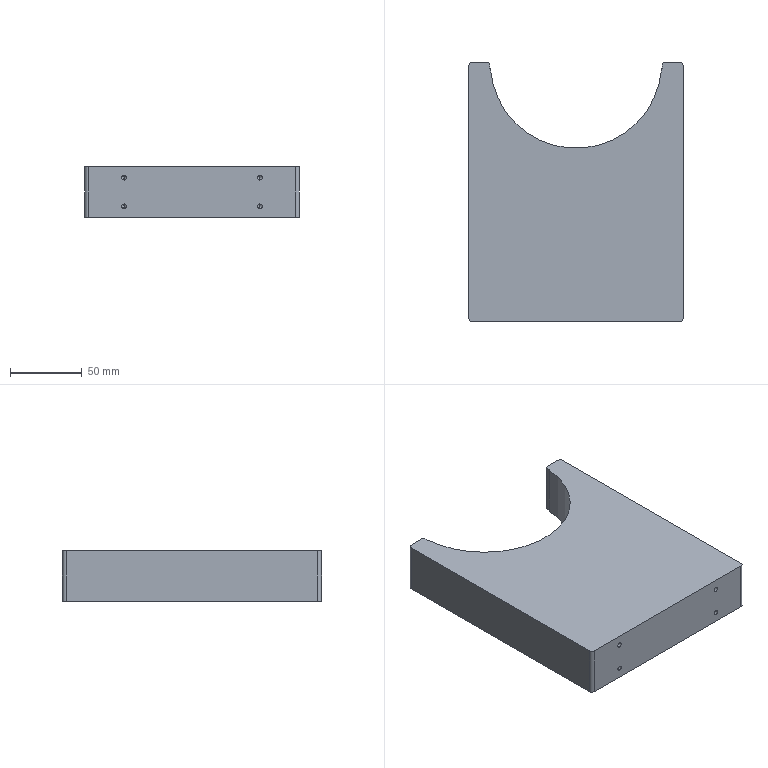Part | SolidWorks | features HoleWzd 2, ICE 2, Chamfer 1, Extrusion 1, Fillet 1 | 1 solid | 42 faces | box 150 x 181 x 35 mm | volume 751527 mm3 | cylinder 19 | cone 12 | plane 11 | commonest cylinder face diameters 3.3 x12 5 x4 120.9 x2 119.9 x1
STEP:
#1=CARTESIAN_POINT('',(-47.5,-75.5,11.65));
#2=VERTEX_POINT('',#1);
#3=CARTESIAN_POINT('',(-47.5,-75.5,8.35));
#4=VERTEX_POINT('',#3);
#5=CARTESIAN_POINT('',(-47.5,-75.5,10.));
#6=DIRECTION('',(0.,-1.,0.));
#7=DIRECTION('',(0.,0.,-1.));
#8=AXIS2_PLACEMENT_3D('',#5,#6,#7);
#9=CIRCLE('',#8,1.65);
#10=EDGE_CURVE('',#2,#4,#9,.T.);
#11=ORIENTED_EDGE('',*,*,#10,.F.);
#12=CARTESIAN_POINT('',(-47.5,-90.5,11.65));
#13=VERTEX_POINT('',#12);
#14=CARTESIAN_POINT('',(-47.5,-90.5,11.65));
#15=DIRECTION('',(0.,-1.,0.));
#16=VECTOR('',#15,1000.);
#17=LINE('',#14,#16);
#18=EDGE_CURVE('',#2,#13,#17,.T.);
#19=ORIENTED_EDGE('',*,*,#18,.T.);
#20=CARTESIAN_POINT('',(-47.5,-90.5,8.35));
#21=VERTEX_POINT('',#20);
#22=CARTESIAN_POINT('',(-47.5,-90.5,10.));
#23=DIRECTION('',(0.,-1.,0.));
#24=DIRECTION('',(0.,0.,-1.));
#25=AXIS2_PLACEMENT_3D('',#22,#23,#24);
#26=CIRCLE('',#25,1.65);
#27=EDGE_CURVE('',#13,#21,#26,.T.);
#28=ORIENTED_EDGE('',*,*,#27,.T.);
#29=CARTESIAN_POINT('',(-47.5,-90.5,8.35));
#30=DIRECTION('',(0.,-1.,0.));
#31=VECTOR('',#30,1000.);
#32=LINE('',#29,#31);
#33=EDGE_CURVE('',#4,#21,#32,.T.);
#34=ORIENTED_EDGE('',*,*,#33,.F.);
#35=EDGE_LOOP('',(#11,#19,#28,#34));
#36=FACE_OUTER_BOUND('',#35,.T.);
#37=CARTESIAN_POINT('',(-47.5,-90.5,10.));
#38=DIRECTION('',(0.,-1.,0.));
#39=DIRECTION('',(0.,0.,-1.));
#40=AXIS2_PLACEMENT_3D('',#37,#38,#39);
#41=CYLINDRICAL_SURFACE('',#40,1.65);
#42=ADVANCED_FACE('',(#36),#41,.F.);
#43=CARTESIAN_POINT('',(-47.5,-74.509,10.));
#44=VERTEX_POINT('',#43);
#45=CARTESIAN_POINT('',(-47.5,-75.5,8.35));
#46=DIRECTION('',(0.,-0.515,-0.8572));
#47=VECTOR('',#46,1000.);
#48=LINE('',#45,#47);
#49=EDGE_CURVE('',#44,#4,#48,.T.);
#50=ORIENTED_EDGE('',*,*,#49,.F.);
#51=CARTESIAN_POINT('',(-47.5,-75.5,11.65));
#52=DIRECTION('',(0.,-0.515,0.8572));
#53=VECTOR('',#52,1000.);
#54=LINE('',#51,#53);
#55=EDGE_CURVE('',#44,#2,#54,.T.);
#56=ORIENTED_EDGE('',*,*,#55,.T.);
#57=ORIENTED_EDGE('',*,*,#10,.T.);
#58=EDGE_LOOP('',(#50,#56,#57));
#59=FACE_OUTER_BOUND('',#58,.T.);
#60=CARTESIAN_POINT('',(-47.5,-75.5,10.));
#61=DIRECTION('',(0.,-1.,0.));
#62=DIRECTION('',(0.,0.,-1.));
#63=AXIS2_PLACEMENT_3D('',#60,#61,#62);
#64=CONICAL_SURFACE('',#63,1.65,1.03);
#65=ADVANCED_FACE('',(#59),#64,.F.);
#66=CARTESIAN_POINT('',(-47.5,-75.5,-8.35));
#67=VERTEX_POINT('',#66);
#68=CARTESIAN_POINT('',(-47.5,-75.5,-11.65));
#69=VERTEX_POINT('',#68);
#70=CARTESIAN_POINT('',(-47.5,-75.5,-10.));
#71=DIRECTION('',(0.,-1.,0.));
#72=DIRECTION('',(0.,0.,-1.));
#73=AXIS2_PLACEMENT_3D('',#70,#71,#72);
#74=CIRCLE('',#73,1.65);
#75=EDGE_CURVE('',#67,#69,#74,.T.);
#76=ORIENTED_EDGE('',*,*,#75,.F.);
#77=CARTESIAN_POINT('',(-47.5,-90.5,-8.35));
#78=VERTEX_POINT('',#77);
#79=CARTESIAN_POINT('',(-47.5,-90.5,-8.35));
#80=DIRECTION('',(0.,-1.,0.));
#81=VECTOR('',#80,1000.);
#82=LINE('',#79,#81);
#83=EDGE_CURVE('',#67,#78,#82,.T.);
#84=ORIENTED_EDGE('',*,*,#83,.T.);
#85=CARTESIAN_POINT('',(-47.5,-90.5,-11.65));
#86=VERTEX_POINT('',#85);
#87=CARTESIAN_POINT('',(-47.5,-90.5,-10.));
#88=DIRECTION('',(0.,-1.,0.));
#89=DIRECTION('',(0.,0.,-1.));
#90=AXIS2_PLACEMENT_3D('',#87,#88,#89);
#91=CIRCLE('',#90,1.65);
#92=EDGE_CURVE('',#78,#86,#91,.T.);
#93=ORIENTED_EDGE('',*,*,#92,.T.);
#94=CARTESIAN_POINT('',(-47.5,-90.5,-11.65));
#95=DIRECTION('',(0.,-1.,0.));
#96=VECTOR('',#95,1000.);
#97=LINE('',#94,#96);
#98=EDGE_CURVE('',#69,#86,#97,.T.);
#99=ORIENTED_EDGE('',*,*,#98,.F.);
#100=EDGE_LOOP('',(#76,#84,#93,#99));
#101=FACE_OUTER_BOUND('',#100,.T.);
#102=CARTESIAN_POINT('',(-47.5,-90.5,-10.));
#103=DIRECTION('',(0.,-1.,0.));
#104=DIRECTION('',(0.,0.,-1.));
#105=AXIS2_PLACEMENT_3D('',#102,#103,#104);
#106=CYLINDRICAL_SURFACE('',#105,1.65);
#107=ADVANCED_FACE('',(#101),#106,.F.);
#108=CARTESIAN_POINT('',(-47.5,-74.509,-10.));
#109=VERTEX_POINT('',#108);
#110=CARTESIAN_POINT('',(-47.5,-75.5,-11.65));
#111=DIRECTION('',(0.,-0.515,-0.8572));
#112=VECTOR('',#111,1000.);
#113=LINE('',#110,#112);
#114=EDGE_CURVE('',#109,#69,#113,.T.);
#115=ORIENTED_EDGE('',*,*,#114,.F.);
#116=CARTESIAN_POINT('',(-47.5,-75.5,-8.35));
#117=DIRECTION('',(0.,-0.515,0.8572));
#118=VECTOR('',#117,1000.);
#119=LINE('',#116,#118);
#120=EDGE_CURVE('',#109,#67,#119,.T.);
#121=ORIENTED_EDGE('',*,*,#120,.T.);
#122=ORIENTED_EDGE('',*,*,#75,.T.);
#123=EDGE_LOOP('',(#115,#121,#122));
#124=FACE_OUTER_BOUND('',#123,.T.);
#125=CARTESIAN_POINT('',(-47.5,-75.5,-10.));
#126=DIRECTION('',(0.,-1.,0.));
#127=DIRECTION('',(0.,0.,-1.));
#128=AXIS2_PLACEMENT_3D('',#125,#126,#127);
#129=CONICAL_SURFACE('',#128,1.65,1.03);
#130=ADVANCED_FACE('',(#124),#129,.F.);
#131=CARTESIAN_POINT('',(47.5,-75.5,11.65));
#132=VERTEX_POINT('',#131);
#133=CARTESIAN_POINT('',(47.5,-75.5,8.35));
#134=VERTEX_POINT('',#133);
#135=CARTESIAN_POINT('',(47.5,-75.5,10.));
#136=DIRECTION('',(0.,-1.,0.));
#137=DIRECTION('',(0.,0.,-1.));
#138=AXIS2_PLACEMENT_3D('',#135,#136,#137);
#139=CIRCLE('',#138,1.65);
#140=EDGE_CURVE('',#132,#134,#139,.T.);
#141=ORIENTED_EDGE('',*,*,#140,.F.);
#142=CARTESIAN_POINT('',(47.5,-90.5,11.65));
#143=VERTEX_POINT('',#142);
#144=CARTESIAN_POINT('',(47.5,-90.5,11.65));
#145=DIRECTION('',(0.,-1.,0.));
#146=VECTOR('',#145,1000.);
#147=LINE('',#144,#146);
#148=EDGE_CURVE('',#132,#143,#147,.T.);
#149=ORIENTED_EDGE('',*,*,#148,.T.);
#150=CARTESIAN_POINT('',(47.5,-90.5,8.35));
#151=VERTEX_POINT('',#150);
#152=CARTESIAN_POINT('',(47.5,-90.5,10.));
#153=DIRECTION('',(0.,-1.,0.));
#154=DIRECTION('',(0.,0.,-1.));
#155=AXIS2_PLACEMENT_3D('',#152,#153,#154);
#156=CIRCLE('',#155,1.65);
#157=EDGE_CURVE('',#143,#151,#156,.T.);
#158=ORIENTED_EDGE('',*,*,#157,.T.);
#159=CARTESIAN_POINT('',(47.5,-90.5,8.35));
#160=DIRECTION('',(0.,-1.,0.));
#161=VECTOR('',#160,1000.);
#162=LINE('',#159,#161);
#163=EDGE_CURVE('',#134,#151,#162,.T.);
#164=ORIENTED_EDGE('',*,*,#163,.F.);
#165=EDGE_LOOP('',(#141,#149,#158,#164));
#166=FACE_OUTER_BOUND('',#165,.T.);
#167=CARTESIAN_POINT('',(47.5,-90.5,10.));
#168=DIRECTION('',(0.,-1.,0.));
#169=DIRECTION('',(0.,0.,-1.));
#170=AXIS2_PLACEMENT_3D('',#167,#168,#169);
#171=CYLINDRICAL_SURFACE('',#170,1.65);
#172=ADVANCED_FACE('',(#166),#171,.F.);
#173=CARTESIAN_POINT('',(47.5,-74.509,10.));
#174=VERTEX_POINT('',#173);
#175=CARTESIAN_POINT('',(47.5,-75.5,8.35));
#176=DIRECTION('',(0.,-0.515,-0.8572));
#177=VECTOR('',#176,1000.);
#178=LINE('',#175,#177);
#179=EDGE_CURVE('',#174,#134,#178,.T.);
#180=ORIENTED_EDGE('',*,*,#179,.F.);
#181=CARTESIAN_POINT('',(47.5,-75.5,11.65));
#182=DIRECTION('',(0.,-0.515,0.8572));
#183=VECTOR('',#182,1000.);
#184=LINE('',#181,#183);
#185=EDGE_CURVE('',#174,#132,#184,.T.);
#186=ORIENTED_EDGE('',*,*,#185,.T.);
#187=ORIENTED_EDGE('',*,*,#140,.T.);
#188=EDGE_LOOP('',(#180,#186,#187));
#189=FACE_OUTER_BOUND('',#188,.T.);
#190=CARTESIAN_POINT('',(47.5,-75.5,10.));
#191=DIRECTION('',(0.,-1.,0.));
#192=DIRECTION('',(0.,0.,-1.));
#193=AXIS2_PLACEMENT_3D('',#190,#191,#192);
#194=CONICAL_SURFACE('',#193,1.65,1.03);
#195=ADVANCED_FACE('',(#189),#194,.F.);
#196=CARTESIAN_POINT('',(47.5,-75.5,-8.35));
#197=VERTEX_POINT('',#196);
#198=CARTESIAN_POINT('',(47.5,-75.5,-11.65));
#199=VERTEX_POINT('',#198);
#200=CARTESIAN_POINT('',(47.5,-75.5,-10.));
#201=DIRECTION('',(0.,-1.,0.));
#202=DIRECTION('',(0.,0.,-1.));
#203=AXIS2_PLACEMENT_3D('',#200,#201,#202);
#204=CIRCLE('',#203,1.65);
#205=EDGE_CURVE('',#197,#199,#204,.T.);
#206=ORIENTED_EDGE('',*,*,#205,.F.);
#207=CARTESIAN_POINT('',(47.5,-90.5,-8.35));
#208=VERTEX_POINT('',#207);
#209=CARTESIAN_POINT('',(47.5,-90.5,-8.35));
#210=DIRECTION('',(0.,-1.,0.));
#211=VECTOR('',#210,1000.);
#212=LINE('',#209,#211);
#213=EDGE_CURVE('',#197,#208,#212,.T.);
#214=ORIENTED_EDGE('',*,*,#213,.T.);
#215=CARTESIAN_POINT('',(47.5,-90.5,-11.65));
#216=VERTEX_POINT('',#215);
#217=CARTESIAN_POINT('',(47.5,-90.5,-10.));
#218=DIRECTION('',(0.,-1.,0.));
#219=DIRECTION('',(0.,0.,-1.));
#220=AXIS2_PLACEMENT_3D('',#217,#218,#219);
#221=CIRCLE('',#220,1.65);
#222=EDGE_CURVE('',#208,#216,#221,.T.);
#223=ORIENTED_EDGE('',*,*,#222,.T.);
#224=CARTESIAN_POINT('',(47.5,-90.5,-11.65));
#225=DIRECTION('',(0.,-1.,0.));
#226=VECTOR('',#225,1000.);
#227=LINE('',#224,#226);
#228=EDGE_CURVE('',#199,#216,#227,.T.);
#229=ORIENTED_EDGE('',*,*,#228,.F.);
#230=EDGE_LOOP('',(#206,#214,#223,#229));
#231=FACE_OUTER_BOUND('',#230,.T.);
#232=CARTESIAN_POINT('',(47.5,-90.5,-10.));
#233=DIRECTION('',(0.,-1.,0.));
#234=DIRECTION('',(0.,0.,-1.));
#235=AXIS2_PLACEMENT_3D('',#232,#233,#234);
#236=CYLINDRICAL_SURFACE('',#235,1.65);
#237=ADVANCED_FACE('',(#231),#236,.F.);
#238=CARTESIAN_POINT('',(47.5,-74.509,-10.));
#239=VERTEX_POINT('',#238);
#240=CARTESIAN_POINT('',(47.5,-75.5,-11.65));
#241=DIRECTION('',(0.,-0.515,-0.8572));
#242=VECTOR('',#241,1000.);
#243=LINE('',#240,#242);
#244=EDGE_CURVE('',#239,#199,#243,.T.);
#245=ORIENTED_EDGE('',*,*,#244,.F.);
#246=CARTESIAN_POINT('',(47.5,-75.5,-8.35));
#247=DIRECTION('',(0.,-0.515,0.8572));
#248=VECTOR('',#247,1000.);
#249=LINE('',#246,#248);
#250=EDGE_CURVE('',#239,#197,#249,.T.);
#251=ORIENTED_EDGE('',*,*,#250,.T.);
#252=ORIENTED_EDGE('',*,*,#205,.T.);
#253=EDGE_LOOP('',(#245,#251,#252));
#254=FACE_OUTER_BOUND('',#253,.T.);
#255=CARTESIAN_POINT('',(47.5,-75.5,-10.));
#256=DIRECTION('',(0.,-1.,0.));
#257=DIRECTION('',(0.,0.,-1.));
#258=AXIS2_PLACEMENT_3D('',#255,#256,#257);
#259=CONICAL_SURFACE('',#258,1.65,1.03);
#260=ADVANCED_FACE('',(#254),#259,.F.);
#261=CARTESIAN_POINT('',(-69.879,75.5,-1.65));
#262=VERTEX_POINT('',#261);
#263=CARTESIAN_POINT('',(-69.879,75.5,1.65));
#264=VERTEX_POINT('',#263);
#265=CARTESIAN_POINT('',(-69.879,75.5,0.));
#266=DIRECTION('',(0.,1.,0.));
#267=DIRECTION('',(0.,0.,1.));
#268=AXIS2_PLACEMENT_3D('',#265,#266,#267);
#269=CIRCLE('',#268,1.65);
#270=EDGE_CURVE('',#262,#264,#269,.T.);
#271=ORIENTED_EDGE('',*,*,#270,.F.);
#272=CARTESIAN_POINT('',(-69.879,90.5,-1.65));
#273=VERTEX_POINT('',#272);
#274=CARTESIAN_POINT('',(-69.879,90.5,-1.65));
#275=DIRECTION('',(0.,1.,0.));
#276=VECTOR('',#275,1000.);
#277=LINE('',#274,#276);
#278=EDGE_CURVE('',#262,#273,#277,.T.);
#279=ORIENTED_EDGE('',*,*,#278,.T.);
#280=CARTESIAN_POINT('',(-69.879,90.5,1.65));
#281=VERTEX_POINT('',#280);
#282=CARTESIAN_POINT('',(-69.879,90.5,0.));
#283=DIRECTION('',(0.,1.,0.));
#284=DIRECTION('',(0.,0.,1.));
#285=AXIS2_PLACEMENT_3D('',#282,#283,#284);
#286=CIRCLE('',#285,1.65);
#287=EDGE_CURVE('',#273,#281,#286,.T.);
#288=ORIENTED_EDGE('',*,*,#287,.T.);
#289=CARTESIAN_POINT('',(-69.879,90.5,1.65));
#290=DIRECTION('',(0.,1.,0.));
#291=VECTOR('',#290,1000.);
#292=LINE('',#289,#291);
#293=EDGE_CURVE('',#264,#281,#292,.T.);
#294=ORIENTED_EDGE('',*,*,#293,.F.);
#295=EDGE_LOOP('',(#271,#279,#288,#294));
#296=FACE_OUTER_BOUND('',#295,.T.);
#297=CARTESIAN_POINT('',(-69.879,90.5,0.));
#298=DIRECTION('',(0.,1.,0.));
#299=DIRECTION('',(0.,0.,1.));
#300=AXIS2_PLACEMENT_3D('',#297,#298,#299);
#301=CYLINDRICAL_SURFACE('',#300,1.65);
#302=ADVANCED_FACE('',(#296),#301,.F.);
#303=CARTESIAN_POINT('',(-69.879,74.509,0.));
#304=VERTEX_POINT('',#303);
#305=CARTESIAN_POINT('',(-69.879,75.5,1.65));
#306=DIRECTION('',(0.,0.515,0.8572));
#307=VECTOR('',#306,1000.);
#308=LINE('',#305,#307);
#309=EDGE_CURVE('',#304,#264,#308,.T.);
#310=ORIENTED_EDGE('',*,*,#309,.F.);
#311=CARTESIAN_POINT('',(-69.879,75.5,-1.65));
#312=DIRECTION('',(0.,0.515,-0.8572));
#313=VECTOR('',#312,1000.);
#314=LINE('',#311,#313);
#315=EDGE_CURVE('',#304,#262,#314,.T.);
#316=ORIENTED_EDGE('',*,*,#315,.T.);
#317=ORIENTED_EDGE('',*,*,#270,.T.);
#318=EDGE_LOOP('',(#310,#316,#317));
#319=FACE_OUTER_BOUND('',#318,.T.);
#320=CARTESIAN_POINT('',(-69.879,75.5,0.));
#321=DIRECTION('',(0.,1.,0.));
#322=DIRECTION('',(0.,0.,1.));
#323=AXIS2_PLACEMENT_3D('',#320,#321,#322);
#324=CONICAL_SURFACE('',#323,1.65,1.03);
#325=ADVANCED_FACE('',(#319),#324,.F.);
#326=CARTESIAN_POINT('',(69.879,75.5,-1.65));
#327=VERTEX_POINT('',#326);
#328=CARTESIAN_POINT('',(69.879,75.5,1.65));
#329=VERTEX_POINT('',#328);
#330=CARTESIAN_POINT('',(69.879,75.5,0.));
#331=DIRECTION('',(0.,1.,0.));
#332=DIRECTION('',(0.,0.,1.));
#333=AXIS2_PLACEMENT_3D('',#330,#331,#332);
#334=CIRCLE('',#333,1.65);
#335=EDGE_CURVE('',#327,#329,#334,.T.);
#336=ORIENTED_EDGE('',*,*,#335,.F.);
#337=CARTESIAN_POINT('',(69.879,90.5,-1.65));
#338=VERTEX_POINT('',#337);
#339=CARTESIAN_POINT('',(69.879,90.5,-1.65));
#340=DIRECTION('',(0.,1.,0.));
#341=VECTOR('',#340,1000.);
#342=LINE('',#339,#341);
#343=EDGE_CURVE('',#327,#338,#342,.T.);
#344=ORIENTED_EDGE('',*,*,#343,.T.);
#345=CARTESIAN_POINT('',(69.879,90.5,1.65));
#346=VERTEX_POINT('',#345);
#347=CARTESIAN_POINT('',(69.879,90.5,0.));
#348=DIRECTION('',(0.,1.,0.));
#349=DIRECTION('',(0.,0.,1.));
#350=AXIS2_PLACEMENT_3D('',#347,#348,#349);
#351=CIRCLE('',#350,1.65);
#352=EDGE_CURVE('',#338,#346,#351,.T.);
#353=ORIENTED_EDGE('',*,*,#352,.T.);
#354=CARTESIAN_POINT('',(69.879,90.5,1.65));
#355=DIRECTION('',(0.,1.,0.));
#356=VECTOR('',#355,1000.);
#357=LINE('',#354,#356);
#358=EDGE_CURVE('',#329,#346,#357,.T.);
#359=ORIENTED_EDGE('',*,*,#358,.F.);
#360=EDGE_LOOP('',(#336,#344,#353,#359));
#361=FACE_OUTER_BOUND('',#360,.T.);
#362=CARTESIAN_POINT('',(69.879,90.5,0.));
#363=DIRECTION('',(0.,1.,0.));
#364=DIRECTION('',(0.,0.,1.));
#365=AXIS2_PLACEMENT_3D('',#362,#363,#364);
#366=CYLINDRICAL_SURFACE('',#365,1.65);
#367=ADVANCED_FACE('',(#361),#366,.F.);
#368=CARTESIAN_POINT('',(69.879,74.509,0.));
#369=VERTEX_POINT('',#368);
#370=CARTESIAN_POINT('',(69.879,75.5,1.65));
#371=DIRECTION('',(0.,0.515,0.8572));
#372=VECTOR('',#371,1000.);
#373=LINE('',#370,#372);
#374=EDGE_CURVE('',#369,#329,#373,.T.);
#375=ORIENTED_EDGE('',*,*,#374,.F.);
#376=CARTESIAN_POINT('',(69.879,75.5,-1.65));
#377=DIRECTION('',(0.,0.515,-0.8572));
#378=VECTOR('',#377,1000.);
#379=LINE('',#376,#378);
#380=EDGE_CURVE('',#369,#327,#379,.T.);
#381=ORIENTED_EDGE('',*,*,#380,.T.);
#382=ORIENTED_EDGE('',*,*,#335,.T.);
#383=EDGE_LOOP('',(#375,#381,#382));
#384=FACE_OUTER_BOUND('',#383,.T.);
#385=CARTESIAN_POINT('',(69.879,75.5,0.));
#386=DIRECTION('',(0.,1.,0.));
#387=DIRECTION('',(0.,0.,1.));
#388=AXIS2_PLACEMENT_3D('',#385,#386,#387);
#389=CONICAL_SURFACE('',#388,1.65,1.03);
#390=ADVANCED_FACE('',(#384),#389,.F.);
#391=CARTESIAN_POINT('',(69.879,90.5,0.));
#392=DIRECTION('',(0.,1.,0.));
#393=DIRECTION('',(0.,0.,1.));
#394=AXIS2_PLACEMENT_3D('',#391,#392,#393);
#395=CIRCLE('',#394,1.65);
#396=EDGE_CURVE('',#346,#338,#395,.T.);
#397=ORIENTED_EDGE('',*,*,#396,.F.);
#398=ORIENTED_EDGE('',*,*,#352,.F.);
#399=EDGE_LOOP('',(#397,#398));
#400=FACE_BOUND('',#399,.T.);
#401=CARTESIAN_POINT('',(72.5,90.5,17.5));
#402=VERTEX_POINT('',#401);
#403=CARTESIAN_POINT('',(60.95,90.5,17.5));
#404=VERTEX_POINT('',#403);
#405=CARTESIAN_POINT('',(-75.,90.5,17.5));
#406=DIRECTION('',(-1.,0.,0.));
#407=VECTOR('',#406,1000.);
#408=LINE('',#405,#407);
#409=EDGE_CURVE('',#402,#404,#408,.T.);
#410=ORIENTED_EDGE('',*,*,#409,.F.);
#411=CARTESIAN_POINT('',(72.5,90.5,-17.5));
#412=VERTEX_POINT('',#411);
#413=CARTESIAN_POINT('',(72.5,90.5,17.5));
#414=DIRECTION('',(0.,0.,-1.));
#415=VECTOR('',#414,1000.);
#416=LINE('',#413,#415);
#417=EDGE_CURVE('',#402,#412,#416,.T.);
#418=ORIENTED_EDGE('',*,*,#417,.T.);
#419=CARTESIAN_POINT('',(60.95,90.5,-17.5));
#420=VERTEX_POINT('',#419);
#421=CARTESIAN_POINT('',(-75.,90.5,-17.5));
#422=DIRECTION('',(-1.,0.,0.));
#423=VECTOR('',#422,1000.);
#424=LINE('',#421,#423);
#425=EDGE_CURVE('',#412,#420,#424,.T.);
#426=ORIENTED_EDGE('',*,*,#425,.T.);
#427=CARTESIAN_POINT('',(60.95,90.5,17.5));
#428=DIRECTION('',(0.,0.,1.));
#429=VECTOR('',#428,1000.);
#430=LINE('',#427,#429);
#431=EDGE_CURVE('',#420,#404,#430,.T.);
#432=ORIENTED_EDGE('',*,*,#431,.T.);
#433=EDGE_LOOP('',(#410,#418,#426,#432));
#434=FACE_OUTER_BOUND('',#433,.T.);
#435=CARTESIAN_POINT('',(-75.,90.5,17.5));
#436=DIRECTION('',(0.,-1.,0.));
#437=DIRECTION('',(1.,0.,0.));
#438=AXIS2_PLACEMENT_3D('',#435,#436,#437);
#439=PLANE('',#438);
#440=ADVANCED_FACE('',(#400,#434),#439,.F.);
#441=CARTESIAN_POINT('',(75.,-88.,17.5));
#442=VERTEX_POINT('',#441);
#443=CARTESIAN_POINT('',(75.,88.,17.5));
#444=VERTEX_POINT('',#443);
#445=CARTESIAN_POINT('',(75.,90.5,17.5));
#446=DIRECTION('',(0.,1.,0.));
#447=VECTOR('',#446,1000.);
#448=LINE('',#445,#447);
#449=EDGE_CURVE('',#442,#444,#448,.T.);
#450=ORIENTED_EDGE('',*,*,#449,.F.);
#451=CARTESIAN_POINT('',(75.,-88.,-17.5));
#452=VERTEX_POINT('',#451);
#453=CARTESIAN_POINT('',(75.,-88.,17.5));
#454=DIRECTION('',(0.,0.,-1.));
#455=VECTOR('',#454,1000.);
#456=LINE('',#453,#455);
#457=EDGE_CURVE('',#442,#452,#456,.T.);
#458=ORIENTED_EDGE('',*,*,#457,.T.);
#459=CARTESIAN_POINT('',(75.,88.,-17.5));
#460=VERTEX_POINT('',#459);
#461=CARTESIAN_POINT('',(75.,90.5,-17.5));
#462=DIRECTION('',(0.,1.,0.));
#463=VECTOR('',#462,1000.);
#464=LINE('',#461,#463);
#465=EDGE_CURVE('',#452,#460,#464,.T.);
#466=ORIENTED_EDGE('',*,*,#465,.T.);
#467=CARTESIAN_POINT('',(75.,88.,17.5));
#468=DIRECTION('',(0.,0.,1.));
#469=VECTOR('',#468,1000.);
#470=LINE('',#467,#469);
#471=EDGE_CURVE('',#460,#444,#470,.T.);
#472=ORIENTED_EDGE('',*,*,#471,.T.);
#473=EDGE_LOOP('',(#450,#458,#466,#472));
#474=FACE_OUTER_BOUND('',#473,.T.);
#475=CARTESIAN_POINT('',(75.,90.5,17.5));
#476=DIRECTION('',(-1.,0.,0.));
#477=DIRECTION('',(0.,-1.,0.));
#478=AXIS2_PLACEMENT_3D('',#475,#476,#477);
#479=PLANE('',#478);
#480=ADVANCED_FACE('',(#474),#479,.F.);
#481=CARTESIAN_POINT('',(-69.879,90.5,0.));
#482=DIRECTION('',(0.,1.,0.));
#483=DIRECTION('',(0.,0.,1.));
#484=AXIS2_PLACEMENT_3D('',#481,#482,#483);
#485=CIRCLE('',#484,1.65);
#486=EDGE_CURVE('',#281,#273,#485,.T.);
#487=ORIENTED_EDGE('',*,*,#486,.F.);
#488=ORIENTED_EDGE('',*,*,#287,.F.);
#489=EDGE_LOOP('',(#487,#488));
#490=FACE_BOUND('',#489,.T.);
#491=CARTESIAN_POINT('',(-60.95,90.5,-17.5));
#492=VERTEX_POINT('',#491);
#493=CARTESIAN_POINT('',(-72.5,90.5,-17.5));
#494=VERTEX_POINT('',#493);
#495=CARTESIAN_POINT('',(-75.,90.5,-17.5));
#496=DIRECTION('',(-1.,0.,0.));
#497=VECTOR('',#496,1000.);
#498=LINE('',#495,#497);
#499=EDGE_CURVE('',#492,#494,#498,.T.);
#500=ORIENTED_EDGE('',*,*,#499,.T.);
#501=CARTESIAN_POINT('',(-72.5,90.5,17.5));
#502=VERTEX_POINT('',#501);
#503=CARTESIAN_POINT('',(-72.5,90.5,17.5));
#504=DIRECTION('',(0.,0.,1.));
#505=VECTOR('',#504,1000.);
#506=LINE('',#503,#505);
#507=EDGE_CURVE('',#494,#502,#506,.T.);
#508=ORIENTED_EDGE('',*,*,#507,.T.);
#509=CARTESIAN_POINT('',(-60.95,90.5,17.5));
#510=VERTEX_POINT('',#509);
#511=CARTESIAN_POINT('',(-75.,90.5,17.5));
#512=DIRECTION('',(-1.,0.,0.));
#513=VECTOR('',#512,1000.);
#514=LINE('',#511,#513);
#515=EDGE_CURVE('',#510,#502,#514,.T.);
#516=ORIENTED_EDGE('',*,*,#515,.F.);
#517=CARTESIAN_POINT('',(-60.95,90.5,17.5));
#518=DIRECTION('',(0.,0.,-1.));
#519=VECTOR('',#518,1000.);
#520=LINE('',#517,#519);
#521=EDGE_CURVE('',#510,#492,#520,.T.);
#522=ORIENTED_EDGE('',*,*,#521,.T.);
#523=EDGE_LOOP('',(#500,#508,#516,#522));
#524=FACE_OUTER_BOUND('',#523,.T.);
#525=CARTESIAN_POINT('',(-75.,90.5,17.5));
#526=DIRECTION('',(0.,-1.,0.));
#527=DIRECTION('',(1.,0.,0.));
#528=AXIS2_PLACEMENT_3D('',#525,#526,#527);
#529=PLANE('',#528);
#530=ADVANCED_FACE('',(#490,#524),#529,.F.);
#531=CARTESIAN_POINT('',(-75.,88.,-17.5));
#532=VERTEX_POINT('',#531);
#533=CARTESIAN_POINT('',(-75.,-88.,-17.5));
#534=VERTEX_POINT('',#533);
#535=CARTESIAN_POINT('',(-75.,90.5,-17.5));
#536=DIRECTION('',(0.,-1.,0.));
#537=VECTOR('',#536,1000.);
#538=LINE('',#535,#537);
#539=EDGE_CURVE('',#532,#534,#538,.T.);
#540=ORIENTED_EDGE('',*,*,#539,.T.);
#541=CARTESIAN_POINT('',(-75.,-88.,17.5));
#542=VERTEX_POINT('',#541);
#543=CARTESIAN_POINT('',(-75.,-88.,17.5));
#544=DIRECTION('',(0.,0.,1.));
#545=VECTOR('',#544,1000.);
#546=LINE('',#543,#545);
#547=EDGE_CURVE('',#534,#542,#546,.T.);
#548=ORIENTED_EDGE('',*,*,#547,.T.);
#549=CARTESIAN_POINT('',(-75.,88.,17.5));
#550=VERTEX_POINT('',#549);
#551=CARTESIAN_POINT('',(-75.,90.5,17.5));
#552=DIRECTION('',(0.,-1.,0.));
#553=VECTOR('',#552,1000.);
#554=LINE('',#551,#553);
#555=EDGE_CURVE('',#550,#542,#554,.T.);
#556=ORIENTED_EDGE('',*,*,#555,.F.);
#557=CARTESIAN_POINT('',(-75.,88.,17.5));
#558=DIRECTION('',(0.,0.,-1.));
#559=VECTOR('',#558,1000.);
#560=LINE('',#557,#559);
#561=EDGE_CURVE('',#550,#532,#560,.T.);
#562=ORIENTED_EDGE('',*,*,#561,.T.);
#563=EDGE_LOOP('',(#540,#548,#556,#562));
#564=FACE_OUTER_BOUND('',#563,.T.);
#565=CARTESIAN_POINT('',(-75.,90.5,17.5));
#566=DIRECTION('',(1.,0.,0.));
#567=DIRECTION('',(0.,1.,0.));
#568=AXIS2_PLACEMENT_3D('',#565,#566,#567);
#569=PLANE('',#568);
#570=ADVANCED_FACE('',(#564),#569,.F.);
#571=CARTESIAN_POINT('',(-47.5,-90.5,10.));
#572=DIRECTION('',(0.,-1.,0.));
#573=DIRECTION('',(0.,0.,-1.));
#574=AXIS2_PLACEMENT_3D('',#571,#572,#573);
#575=CIRCLE('',#574,1.65);
#576=EDGE_CURVE('',#21,#13,#575,.T.);
#577=ORIENTED_EDGE('',*,*,#576,.F.);
#578=ORIENTED_EDGE('',*,*,#27,.F.);
#579=EDGE_LOOP('',(#577,#578));
#580=FACE_BOUND('',#579,.T.);
#581=CARTESIAN_POINT('',(-47.5,-90.5,-10.));
#582=DIRECTION('',(0.,-1.,0.));
#583=DIRECTION('',(0.,0.,-1.));
#584=AXIS2_PLACEMENT_3D('',#581,#582,#583);
#585=CIRCLE('',#584,1.65);
#586=EDGE_CURVE('',#86,#78,#585,.T.);
#587=ORIENTED_EDGE('',*,*,#586,.F.);
#588=ORIENTED_EDGE('',*,*,#92,.F.);
#589=EDGE_LOOP('',(#587,#588));
#590=FACE_BOUND('',#589,.T.);
#591=CARTESIAN_POINT('',(47.5,-90.5,10.));
#592=DIRECTION('',(0.,-1.,0.));
#593=DIRECTION('',(0.,0.,-1.));
#594=AXIS2_PLACEMENT_3D('',#591,#592,#593);
#595=CIRCLE('',#594,1.65);
#596=EDGE_CURVE('',#151,#143,#595,.T.);
#597=ORIENTED_EDGE('',*,*,#596,.F.);
#598=ORIENTED_EDGE('',*,*,#157,.F.);
#599=EDGE_LOOP('',(#597,#598));
#600=FACE_BOUND('',#599,.T.);
#601=CARTESIAN_POINT('',(47.5,-90.5,-10.));
#602=DIRECTION('',(0.,-1.,0.));
#603=DIRECTION('',(0.,0.,-1.));
#604=AXIS2_PLACEMENT_3D('',#601,#602,#603);
#605=CIRCLE('',#604,1.65);
#606=EDGE_CURVE('',#216,#208,#605,.T.);
#607=ORIENTED_EDGE('',*,*,#606,.F.);
#608=ORIENTED_EDGE('',*,*,#222,.F.);
#609=EDGE_LOOP('',(#607,#608));
#610=FACE_BOUND('',#609,.T.);
#611=CARTESIAN_POINT('',(-72.5,-90.5,-17.5));
#612=VERTEX_POINT('',#611);
#613=CARTESIAN_POINT('',(72.5,-90.5,-17.5));
#614=VERTEX_POINT('',#613);
#615=CARTESIAN_POINT('',(-75.,-90.5,-17.5));
#616=DIRECTION('',(1.,0.,0.));
#617=VECTOR('',#616,1000.);
#618=LINE('',#615,#617);
#619=EDGE_CURVE('',#612,#614,#618,.T.);
#620=ORIENTED_EDGE('',*,*,#619,.T.);
#621=CARTESIAN_POINT('',(72.5,-90.5,17.5));
#622=VERTEX_POINT('',#621);
#623=CARTESIAN_POINT('',(72.5,-90.5,17.5));
#624=DIRECTION('',(0.,0.,1.));
#625=VECTOR('',#624,1000.);
#626=LINE('',#623,#625);
#627=EDGE_CURVE('',#614,#622,#626,.T.);
#628=ORIENTED_EDGE('',*,*,#627,.T.);
#629=CARTESIAN_POINT('',(-72.5,-90.5,17.5));
#630=VERTEX_POINT('',#629);
#631=CARTESIAN_POINT('',(-75.,-90.5,17.5));
#632=DIRECTION('',(1.,0.,0.));
#633=VECTOR('',#632,1000.);
#634=LINE('',#631,#633);
#635=EDGE_CURVE('',#630,#622,#634,.T.);
#636=ORIENTED_EDGE('',*,*,#635,.F.);
#637=CARTESIAN_POINT('',(-72.5,-90.5,17.5));
#638=DIRECTION('',(0.,0.,-1.));
#639=VECTOR('',#638,1000.);
#640=LINE('',#637,#639);
#641=EDGE_CURVE('',#630,#612,#640,.T.);
#642=ORIENTED_EDGE('',*,*,#641,.T.);
#643=EDGE_LOOP('',(#620,#628,#636,#642));
#644=FACE_OUTER_BOUND('',#643,.T.);
#645=CARTESIAN_POINT('',(-75.,-90.5,17.5));
#646=DIRECTION('',(0.,1.,0.));
#647=DIRECTION('',(0.,0.,1.));
#648=AXIS2_PLACEMENT_3D('',#645,#646,#647);
#649=PLANE('',#648);
#650=ADVANCED_FACE('',(#580,#590,#600,#610,#644),#649,.F.);
#651=ORIENTED_EDGE('',*,*,#635,.T.);
#652=CARTESIAN_POINT('',(72.5,-88.,17.5));
#653=DIRECTION('',(0.,0.,1.));
#654=DIRECTION('',(1.,0.,0.));
#655=AXIS2_PLACEMENT_3D('',#652,#653,#654);
#656=CIRCLE('',#655,2.5);
#657=EDGE_CURVE('',#622,#442,#656,.T.);
#658=ORIENTED_EDGE('',*,*,#657,.T.);
#659=ORIENTED_EDGE('',*,*,#449,.T.);
#660=CARTESIAN_POINT('',(72.5,88.,17.5));
#661=DIRECTION('',(0.,0.,1.));
#662=DIRECTION('',(1.,0.,0.));
#663=AXIS2_PLACEMENT_3D('',#660,#661,#662);
#664=CIRCLE('',#663,2.5);
#665=EDGE_CURVE('',#444,#402,#664,.T.);
#666=ORIENTED_EDGE('',*,*,#665,.T.);
#667=ORIENTED_EDGE('',*,*,#409,.T.);
#668=CARTESIAN_POINT('',(60.448,89.998,17.5));
#669=VERTEX_POINT('',#668);
#670=CARTESIAN_POINT('',(-14.775,14.775,17.5));
#671=DIRECTION('',(-0.7071,-0.7071,0.));
#672=VECTOR('',#671,1000.);
#673=LINE('',#670,#672);
#674=EDGE_CURVE('',#404,#669,#673,.T.);
#675=ORIENTED_EDGE('',*,*,#674,.T.);
#676=CARTESIAN_POINT('',(60.315,86.469,17.5));
#677=VERTEX_POINT('',#676);
#678=CARTESIAN_POINT('',(0.,90.5,17.5));
#679=DIRECTION('',(0.,0.,1.));
#680=DIRECTION('',(1.,0.,0.));
#681=AXIS2_PLACEMENT_3D('',#678,#679,#680);
#682=CIRCLE('',#681,60.45);
#683=EDGE_CURVE('',#677,#669,#682,.T.);
#684=ORIENTED_EDGE('',*,*,#683,.F.);
#685=CARTESIAN_POINT('',(59.781,86.006,17.5));
#686=VERTEX_POINT('',#685);
#687=CARTESIAN_POINT('',(-16.918,19.516,17.5));
#688=DIRECTION('',(-0.7556,-0.655,0.));
#689=VECTOR('',#688,1000.);
#690=LINE('',#687,#689);
#691=EDGE_CURVE('',#677,#686,#690,.T.);
#692=ORIENTED_EDGE('',*,*,#691,.T.);
#693=CARTESIAN_POINT('',(-59.781,86.006,17.5));
#694=VERTEX_POINT('',#693);
#695=CARTESIAN_POINT('',(0.,90.5,17.5));
#696=DIRECTION('',(0.,0.,1.));
#697=DIRECTION('',(1.,0.,0.));
#698=AXIS2_PLACEMENT_3D('',#695,#696,#697);
#699=CIRCLE('',#698,59.95);
#700=EDGE_CURVE('',#694,#686,#699,.T.);
#701=ORIENTED_EDGE('',*,*,#700,.F.);
#702=CARTESIAN_POINT('',(-60.315,86.469,17.5));
#703=VERTEX_POINT('',#702);
#704=CARTESIAN_POINT('',(16.918,19.516,17.5));
#705=DIRECTION('',(-0.7556,0.655,0.));
#706=VECTOR('',#705,1000.);
#707=LINE('',#704,#706);
#708=EDGE_CURVE('',#694,#703,#707,.T.);
#709=ORIENTED_EDGE('',*,*,#708,.T.);
#710=CARTESIAN_POINT('',(-60.448,89.998,17.5));
#711=VERTEX_POINT('',#710);
#712=CARTESIAN_POINT('',(0.,90.5,17.5));
#713=DIRECTION('',(0.,0.,1.));
#714=DIRECTION('',(1.,0.,0.));
#715=AXIS2_PLACEMENT_3D('',#712,#713,#714);
#716=CIRCLE('',#715,60.45);
#717=EDGE_CURVE('',#711,#703,#716,.T.);
#718=ORIENTED_EDGE('',*,*,#717,.F.);
#719=CARTESIAN_POINT('',(14.775,14.775,17.5));
#720=DIRECTION('',(-0.7071,0.7071,0.));
#721=VECTOR('',#720,1000.);
#722=LINE('',#719,#721);
#723=EDGE_CURVE('',#711,#510,#722,.T.);
#724=ORIENTED_EDGE('',*,*,#723,.T.);
#725=ORIENTED_EDGE('',*,*,#515,.T.);
#726=CARTESIAN_POINT('',(-72.5,88.,17.5));
#727=DIRECTION('',(0.,0.,1.));
#728=DIRECTION('',(1.,0.,0.));
#729=AXIS2_PLACEMENT_3D('',#726,#727,#728);
#730=CIRCLE('',#729,2.5);
#731=EDGE_CURVE('',#502,#550,#730,.T.);
#732=ORIENTED_EDGE('',*,*,#731,.T.);
#733=ORIENTED_EDGE('',*,*,#555,.T.);
#734=CARTESIAN_POINT('',(-72.5,-88.,17.5));
#735=DIRECTION('',(0.,0.,1.));
#736=DIRECTION('',(1.,0.,0.));
#737=AXIS2_PLACEMENT_3D('',#734,#735,#736);
#738=CIRCLE('',#737,2.5);
#739=EDGE_CURVE('',#542,#630,#738,.T.);
#740=ORIENTED_EDGE('',*,*,#739,.T.);
#741=EDGE_LOOP('',(#651,#658,#659,#666,#667,#675,#684,#692,#701,#709,#718,#724,#725,#732,#733,#740));
#742=FACE_OUTER_BOUND('',#741,.T.);
#743=CARTESIAN_POINT('',(0.,0.,17.5));
#744=DIRECTION('',(0.,0.,1.));
#745=DIRECTION('',(1.,0.,0.));
#746=AXIS2_PLACEMENT_3D('',#743,#744,#745);
#747=PLANE('',#746);
#748=ADVANCED_FACE('',(#742),#747,.T.);
#749=ORIENTED_EDGE('',*,*,#465,.F.);
#750=CARTESIAN_POINT('',(72.5,-88.,-17.5));
#751=DIRECTION('',(0.,0.,-1.));
#752=DIRECTION('',(1.,0.,0.));
#753=AXIS2_PLACEMENT_3D('',#750,#751,#752);
#754=CIRCLE('',#753,2.5);
#755=EDGE_CURVE('',#452,#614,#754,.T.);
#756=ORIENTED_EDGE('',*,*,#755,.T.);
#757=ORIENTED_EDGE('',*,*,#619,.F.);
#758=CARTESIAN_POINT('',(-72.5,-88.,-17.5));
#759=DIRECTION('',(0.,0.,-1.));
#760=DIRECTION('',(1.,0.,0.));
#761=AXIS2_PLACEMENT_3D('',#758,#759,#760);
#762=CIRCLE('',#761,2.5);
#763=EDGE_CURVE('',#612,#534,#762,.T.);
#764=ORIENTED_EDGE('',*,*,#763,.T.);
#765=ORIENTED_EDGE('',*,*,#539,.F.);
#766=CARTESIAN_POINT('',(-72.5,88.,-17.5));
#767=DIRECTION('',(0.,0.,-1.));
#768=DIRECTION('',(1.,0.,0.));
#769=AXIS2_PLACEMENT_3D('',#766,#767,#768);
#770=CIRCLE('',#769,2.5);
#771=EDGE_CURVE('',#532,#494,#770,.T.);
#772=ORIENTED_EDGE('',*,*,#771,.T.);
#773=ORIENTED_EDGE('',*,*,#499,.F.);
#774=CARTESIAN_POINT('',(-60.448,89.998,-17.5));
#775=VERTEX_POINT('',#774);
#776=CARTESIAN_POINT('',(-60.448,89.998,-17.5));
#777=DIRECTION('',(0.7071,-0.7071,0.));
#778=VECTOR('',#777,1000.);
#779=LINE('',#776,#778);
#780=EDGE_CURVE('',#492,#775,#779,.T.);
#781=ORIENTED_EDGE('',*,*,#780,.T.);
#782=CARTESIAN_POINT('',(-60.315,86.469,-17.5));
#783=VERTEX_POINT('',#782);
#784=CARTESIAN_POINT('',(0.,90.5,-17.5));
#785=DIRECTION('',(0.,0.,1.));
#786=DIRECTION('',(1.,0.,0.));
#787=AXIS2_PLACEMENT_3D('',#784,#785,#786);
#788=CIRCLE('',#787,60.45);
#789=EDGE_CURVE('',#775,#783,#788,.T.);
#790=ORIENTED_EDGE('',*,*,#789,.T.);
#791=CARTESIAN_POINT('',(-59.781,86.006,-17.5));
#792=VERTEX_POINT('',#791);
#793=CARTESIAN_POINT('',(-59.781,86.006,-17.5));
#794=DIRECTION('',(0.7556,-0.655,0.));
#795=VECTOR('',#794,1000.);
#796=LINE('',#793,#795);
#797=EDGE_CURVE('',#783,#792,#796,.T.);
#798=ORIENTED_EDGE('',*,*,#797,.T.);
#799=CARTESIAN_POINT('',(59.781,86.006,-17.5));
#800=VERTEX_POINT('',#799);
#801=CARTESIAN_POINT('',(0.,90.5,-17.5));
#802=DIRECTION('',(0.,0.,1.));
#803=DIRECTION('',(1.,0.,0.));
#804=AXIS2_PLACEMENT_3D('',#801,#802,#803);
#805=CIRCLE('',#804,59.95);
#806=EDGE_CURVE('',#792,#800,#805,.T.);
#807=ORIENTED_EDGE('',*,*,#806,.T.);
#808=CARTESIAN_POINT('',(60.315,86.469,-17.5));
#809=VERTEX_POINT('',#808);
#810=CARTESIAN_POINT('',(60.351,86.5,-17.5));
#811=DIRECTION('',(0.7556,0.655,0.));
#812=VECTOR('',#811,1000.);
#813=LINE('',#810,#812);
#814=EDGE_CURVE('',#800,#809,#813,.T.);
#815=ORIENTED_EDGE('',*,*,#814,.T.);
#816=CARTESIAN_POINT('',(60.448,89.998,-17.5));
#817=VERTEX_POINT('',#816);
#818=CARTESIAN_POINT('',(0.,90.5,-17.5));
#819=DIRECTION('',(0.,0.,1.));
#820=DIRECTION('',(1.,0.,0.));
#821=AXIS2_PLACEMENT_3D('',#818,#819,#820);
#822=CIRCLE('',#821,60.45);
#823=EDGE_CURVE('',#809,#817,#822,.T.);
#824=ORIENTED_EDGE('',*,*,#823,.T.);
#825=CARTESIAN_POINT('',(60.95,90.5,-17.5));
#826=DIRECTION('',(0.7071,0.7071,0.));
#827=VECTOR('',#826,1000.);
#828=LINE('',#825,#827);
#829=EDGE_CURVE('',#817,#420,#828,.T.);
#830=ORIENTED_EDGE('',*,*,#829,.T.);
#831=ORIENTED_EDGE('',*,*,#425,.F.);
#832=CARTESIAN_POINT('',(72.5,88.,-17.5));
#833=DIRECTION('',(0.,0.,-1.));
#834=DIRECTION('',(1.,0.,0.));
#835=AXIS2_PLACEMENT_3D('',#832,#833,#834);
#836=CIRCLE('',#835,2.5);
#837=EDGE_CURVE('',#412,#460,#836,.T.);
#838=ORIENTED_EDGE('',*,*,#837,.T.);
#839=EDGE_LOOP('',(#749,#756,#757,#764,#765,#772,#773,#781,#790,#798,#807,#815,#824,#830,#831,#838));
#840=FACE_OUTER_BOUND('',#839,.T.);
#841=CARTESIAN_POINT('',(0.,0.,-17.5));
#842=DIRECTION('',(0.,0.,1.));
#843=DIRECTION('',(1.,0.,0.));
#844=AXIS2_PLACEMENT_3D('',#841,#842,#843);
#845=PLANE('',#844);
#846=ADVANCED_FACE('',(#840),#845,.F.);
#847=ORIENTED_EDGE('',*,*,#806,.F.);
#848=CARTESIAN_POINT('',(-59.781,86.006,-50.));
#849=DIRECTION('',(0.,0.,1.));
#850=VECTOR('',#849,1000.);
#851=LINE('',#848,#850);
#852=EDGE_CURVE('',#792,#694,#851,.T.);
#853=ORIENTED_EDGE('',*,*,#852,.T.);
#854=ORIENTED_EDGE('',*,*,#700,.T.);
#855=CARTESIAN_POINT('',(59.781,86.006,-50.));
#856=DIRECTION('',(0.,0.,-1.));
#857=VECTOR('',#856,1000.);
#858=LINE('',#855,#857);
#859=EDGE_CURVE('',#686,#800,#858,.T.);
#860=ORIENTED_EDGE('',*,*,#859,.T.);
#861=EDGE_LOOP('',(#847,#853,#854,#860));
#862=FACE_OUTER_BOUND('',#861,.T.);
#863=CARTESIAN_POINT('',(0.,90.5,-50.));
#864=DIRECTION('',(0.,0.,1.));
#865=DIRECTION('',(1.,0.,0.));
#866=AXIS2_PLACEMENT_3D('',#863,#864,#865);
#867=CYLINDRICAL_SURFACE('',#866,59.95);
#868=ADVANCED_FACE('',(#862),#867,.F.);
#869=ORIENTED_EDGE('',*,*,#683,.T.);
#870=CARTESIAN_POINT('',(60.448,89.998,-17.5));
#871=DIRECTION('',(0.,0.,-1.));
#872=VECTOR('',#871,1000.);
#873=LINE('',#870,#872);
#874=EDGE_CURVE('',#669,#817,#873,.T.);
#875=ORIENTED_EDGE('',*,*,#874,.T.);
#876=ORIENTED_EDGE('',*,*,#823,.F.);
#877=CARTESIAN_POINT('',(60.315,86.469,0.));
#878=DIRECTION('',(0.,0.,1.));
#879=VECTOR('',#878,1000.);
#880=LINE('',#877,#879);
#881=EDGE_CURVE('',#809,#677,#880,.T.);
#882=ORIENTED_EDGE('',*,*,#881,.T.);
#883=EDGE_LOOP('',(#869,#875,#876,#882));
#884=FACE_OUTER_BOUND('',#883,.T.);
#885=CARTESIAN_POINT('',(0.,90.5,-17.5));
#886=DIRECTION('',(0.,0.,1.));
#887=DIRECTION('',(1.,0.,0.));
#888=AXIS2_PLACEMENT_3D('',#885,#886,#887);
#889=CYLINDRICAL_SURFACE('',#888,60.45);
#890=ADVANCED_FACE('',(#884),#889,.F.);
#891=ORIENTED_EDGE('',*,*,#789,.F.);
#892=CARTESIAN_POINT('',(-60.448,89.998,-17.5));
#893=DIRECTION('',(0.,0.,1.));
#894=VECTOR('',#893,1000.);
#895=LINE('',#892,#894);
#896=EDGE_CURVE('',#775,#711,#895,.T.);
#897=ORIENTED_EDGE('',*,*,#896,.T.);
#898=ORIENTED_EDGE('',*,*,#717,.T.);
#899=CARTESIAN_POINT('',(-60.315,86.469,0.));
#900=DIRECTION('',(0.,0.,-1.));
#901=VECTOR('',#900,1000.);
#902=LINE('',#899,#901);
#903=EDGE_CURVE('',#703,#783,#902,.T.);
#904=ORIENTED_EDGE('',*,*,#903,.T.);
#905=EDGE_LOOP('',(#891,#897,#898,#904));
#906=FACE_OUTER_BOUND('',#905,.T.);
#907=CARTESIAN_POINT('',(0.,90.5,-17.5));
#908=DIRECTION('',(0.,0.,1.));
#909=DIRECTION('',(1.,0.,0.));
#910=AXIS2_PLACEMENT_3D('',#907,#908,#909);
#911=CYLINDRICAL_SURFACE('',#910,60.45);
#912=ADVANCED_FACE('',(#906),#911,.F.);
#913=ORIENTED_EDGE('',*,*,#797,.F.);
#914=ORIENTED_EDGE('',*,*,#903,.F.);
#915=ORIENTED_EDGE('',*,*,#708,.F.);
#916=ORIENTED_EDGE('',*,*,#852,.F.);
#917=EDGE_LOOP('',(#913,#914,#915,#916));
#918=FACE_OUTER_BOUND('',#917,.T.);
#919=CARTESIAN_POINT('',(-59.781,86.006,-50.));
#920=DIRECTION('',(-0.655,-0.7556,0.));
#921=DIRECTION('',(0.,0.,1.));
#922=AXIS2_PLACEMENT_3D('',#919,#920,#921);
#923=PLANE('',#922);
#924=ADVANCED_FACE('',(#918),#923,.F.);
#925=ORIENTED_EDGE('',*,*,#829,.F.);
#926=ORIENTED_EDGE('',*,*,#874,.F.);
#927=ORIENTED_EDGE('',*,*,#674,.F.);
#928=ORIENTED_EDGE('',*,*,#431,.F.);
#929=EDGE_LOOP('',(#925,#926,#927,#928));
#930=FACE_OUTER_BOUND('',#929,.T.);
#931=CARTESIAN_POINT('',(60.95,90.5,-17.5));
#932=DIRECTION('',(0.7071,-0.7071,0.));
#933=DIRECTION('',(0.,0.,1.));
#934=AXIS2_PLACEMENT_3D('',#931,#932,#933);
#935=PLANE('',#934);
#936=ADVANCED_FACE('',(#930),#935,.F.);
#937=ORIENTED_EDGE('',*,*,#814,.F.);
#938=ORIENTED_EDGE('',*,*,#859,.F.);
#939=ORIENTED_EDGE('',*,*,#691,.F.);
#940=ORIENTED_EDGE('',*,*,#881,.F.);
#941=EDGE_LOOP('',(#937,#938,#939,#940));
#942=FACE_OUTER_BOUND('',#941,.T.);
#943=CARTESIAN_POINT('',(60.351,86.5,-50.));
#944=DIRECTION('',(0.655,-0.7556,0.));
#945=DIRECTION('',(0.,0.,1.));
#946=AXIS2_PLACEMENT_3D('',#943,#944,#945);
#947=PLANE('',#946);
#948=ADVANCED_FACE('',(#942),#947,.F.);
#949=ORIENTED_EDGE('',*,*,#780,.F.);
#950=ORIENTED_EDGE('',*,*,#521,.F.);
#951=ORIENTED_EDGE('',*,*,#723,.F.);
#952=ORIENTED_EDGE('',*,*,#896,.F.);
#953=EDGE_LOOP('',(#949,#950,#951,#952));
#954=FACE_OUTER_BOUND('',#953,.T.);
#955=CARTESIAN_POINT('',(-60.448,89.998,-17.5));
#956=DIRECTION('',(-0.7071,-0.7071,0.));
#957=DIRECTION('',(0.,0.,1.));
#958=AXIS2_PLACEMENT_3D('',#955,#956,#957);
#959=PLANE('',#958);
#960=ADVANCED_FACE('',(#954),#959,.F.);
#961=ORIENTED_EDGE('',*,*,#380,.F.);
#962=ORIENTED_EDGE('',*,*,#374,.T.);
#963=CARTESIAN_POINT('',(69.879,75.5,0.));
#964=DIRECTION('',(0.,1.,0.));
#965=DIRECTION('',(0.,0.,1.));
#966=AXIS2_PLACEMENT_3D('',#963,#964,#965);
#967=CIRCLE('',#966,1.65);
#968=EDGE_CURVE('',#329,#327,#967,.T.);
#969=ORIENTED_EDGE('',*,*,#968,.T.);
#970=EDGE_LOOP('',(#961,#962,#969));
#971=FACE_OUTER_BOUND('',#970,.T.);
#972=CARTESIAN_POINT('',(69.879,75.5,0.));
#973=DIRECTION('',(0.,1.,0.));
#974=DIRECTION('',(0.,0.,1.));
#975=AXIS2_PLACEMENT_3D('',#972,#973,#974);
#976=CONICAL_SURFACE('',#975,1.65,1.03);
#977=ADVANCED_FACE('',(#971),#976,.F.);
#978=ORIENTED_EDGE('',*,*,#343,.F.);
#979=ORIENTED_EDGE('',*,*,#968,.F.);
#980=ORIENTED_EDGE('',*,*,#358,.T.);
#981=ORIENTED_EDGE('',*,*,#396,.T.);
#982=EDGE_LOOP('',(#978,#979,#980,#981));
#983=FACE_OUTER_BOUND('',#982,.T.);
#984=CARTESIAN_POINT('',(69.879,90.5,0.));
#985=DIRECTION('',(0.,1.,0.));
#986=DIRECTION('',(0.,0.,1.));
#987=AXIS2_PLACEMENT_3D('',#984,#985,#986);
#988=CYLINDRICAL_SURFACE('',#987,1.65);
#989=ADVANCED_FACE('',(#983),#988,.F.);
#990=ORIENTED_EDGE('',*,*,#315,.F.);
#991=ORIENTED_EDGE('',*,*,#309,.T.);
#992=CARTESIAN_POINT('',(-69.879,75.5,0.));
#993=DIRECTION('',(0.,1.,0.));
#994=DIRECTION('',(0.,0.,1.));
#995=AXIS2_PLACEMENT_3D('',#992,#993,#994);
#996=CIRCLE('',#995,1.65);
#997=EDGE_CURVE('',#264,#262,#996,.T.);
#998=ORIENTED_EDGE('',*,*,#997,.T.);
#999=EDGE_LOOP('',(#990,#991,#998));
#1000=FACE_OUTER_BOUND('',#999,.T.);
#1001=CARTESIAN_POINT('',(-69.879,75.5,0.));
#1002=DIRECTION('',(0.,1.,0.));
#1003=DIRECTION('',(0.,0.,1.));
#1004=AXIS2_PLACEMENT_3D('',#1001,#1002,#1003);
#1005=CONICAL_SURFACE('',#1004,1.65,1.03);
#1006=ADVANCED_FACE('',(#1000),#1005,.F.);
#1007=ORIENTED_EDGE('',*,*,#278,.F.);
#1008=ORIENTED_EDGE('',*,*,#997,.F.);
#1009=ORIENTED_EDGE('',*,*,#293,.T.);
#1010=ORIENTED_EDGE('',*,*,#486,.T.);
#1011=EDGE_LOOP('',(#1007,#1008,#1009,#1010));
#1012=FACE_OUTER_BOUND('',#1011,.T.);
#1013=CARTESIAN_POINT('',(-69.879,90.5,0.));
#1014=DIRECTION('',(0.,1.,0.));
#1015=DIRECTION('',(0.,0.,1.));
#1016=AXIS2_PLACEMENT_3D('',#1013,#1014,#1015);
#1017=CYLINDRICAL_SURFACE('',#1016,1.65);
#1018=ADVANCED_FACE('',(#1012),#1017,.F.);
#1019=ORIENTED_EDGE('',*,*,#250,.F.);
#1020=ORIENTED_EDGE('',*,*,#244,.T.);
#1021=CARTESIAN_POINT('',(47.5,-75.5,-10.));
#1022=DIRECTION('',(0.,-1.,0.));
#1023=DIRECTION('',(0.,0.,-1.));
#1024=AXIS2_PLACEMENT_3D('',#1021,#1022,#1023);
#1025=CIRCLE('',#1024,1.65);
#1026=EDGE_CURVE('',#199,#197,#1025,.T.);
#1027=ORIENTED_EDGE('',*,*,#1026,.T.);
#1028=EDGE_LOOP('',(#1019,#1020,#1027));
#1029=FACE_OUTER_BOUND('',#1028,.T.);
#1030=CARTESIAN_POINT('',(47.5,-75.5,-10.));
#1031=DIRECTION('',(0.,-1.,0.));
#1032=DIRECTION('',(0.,0.,-1.));
#1033=AXIS2_PLACEMENT_3D('',#1030,#1031,#1032);
#1034=CONICAL_SURFACE('',#1033,1.65,1.03);
#1035=ADVANCED_FACE('',(#1029),#1034,.F.);
#1036=ORIENTED_EDGE('',*,*,#213,.F.);
#1037=ORIENTED_EDGE('',*,*,#1026,.F.);
#1038=ORIENTED_EDGE('',*,*,#228,.T.);
#1039=ORIENTED_EDGE('',*,*,#606,.T.);
#1040=EDGE_LOOP('',(#1036,#1037,#1038,#1039));
#1041=FACE_OUTER_BOUND('',#1040,.T.);
#1042=CARTESIAN_POINT('',(47.5,-90.5,-10.));
#1043=DIRECTION('',(0.,-1.,0.));
#1044=DIRECTION('',(0.,0.,-1.));
#1045=AXIS2_PLACEMENT_3D('',#1042,#1043,#1044);
#1046=CYLINDRICAL_SURFACE('',#1045,1.65);
#1047=ADVANCED_FACE('',(#1041),#1046,.F.);
#1048=ORIENTED_EDGE('',*,*,#185,.F.);
#1049=ORIENTED_EDGE('',*,*,#179,.T.);
#1050=CARTESIAN_POINT('',(47.5,-75.5,10.));
#1051=DIRECTION('',(0.,-1.,0.));
#1052=DIRECTION('',(0.,0.,-1.));
#1053=AXIS2_PLACEMENT_3D('',#1050,#1051,#1052);
#1054=CIRCLE('',#1053,1.65);
#1055=EDGE_CURVE('',#134,#132,#1054,.T.);
#1056=ORIENTED_EDGE('',*,*,#1055,.T.);
#1057=EDGE_LOOP('',(#1048,#1049,#1056));
#1058=FACE_OUTER_BOUND('',#1057,.T.);
#1059=CARTESIAN_POINT('',(47.5,-75.5,10.));
#1060=DIRECTION('',(0.,-1.,0.));
#1061=DIRECTION('',(0.,0.,-1.));
#1062=AXIS2_PLACEMENT_3D('',#1059,#1060,#1061);
#1063=CONICAL_SURFACE('',#1062,1.65,1.03);
#1064=ADVANCED_FACE('',(#1058),#1063,.F.);
#1065=ORIENTED_EDGE('',*,*,#148,.F.);
#1066=ORIENTED_EDGE('',*,*,#1055,.F.);
#1067=ORIENTED_EDGE('',*,*,#163,.T.);
#1068=ORIENTED_EDGE('',*,*,#596,.T.);
#1069=EDGE_LOOP('',(#1065,#1066,#1067,#1068));
#1070=FACE_OUTER_BOUND('',#1069,.T.);
#1071=CARTESIAN_POINT('',(47.5,-90.5,10.));
#1072=DIRECTION('',(0.,-1.,0.));
#1073=DIRECTION('',(0.,0.,-1.));
#1074=AXIS2_PLACEMENT_3D('',#1071,#1072,#1073);
#1075=CYLINDRICAL_SURFACE('',#1074,1.65);
#1076=ADVANCED_FACE('',(#1070),#1075,.F.);
#1077=ORIENTED_EDGE('',*,*,#120,.F.);
#1078=ORIENTED_EDGE('',*,*,#114,.T.);
#1079=CARTESIAN_POINT('',(-47.5,-75.5,-10.));
#1080=DIRECTION('',(0.,-1.,0.));
#1081=DIRECTION('',(0.,0.,-1.));
#1082=AXIS2_PLACEMENT_3D('',#1079,#1080,#1081);
#1083=CIRCLE('',#1082,1.65);
#1084=EDGE_CURVE('',#69,#67,#1083,.T.);
#1085=ORIENTED_EDGE('',*,*,#1084,.T.);
#1086=EDGE_LOOP('',(#1077,#1078,#1085));
#1087=FACE_OUTER_BOUND('',#1086,.T.);
#1088=CARTESIAN_POINT('',(-47.5,-75.5,-10.));
#1089=DIRECTION('',(0.,-1.,0.));
#1090=DIRECTION('',(0.,0.,-1.));
#1091=AXIS2_PLACEMENT_3D('',#1088,#1089,#1090);
#1092=CONICAL_SURFACE('',#1091,1.65,1.03);
#1093=ADVANCED_FACE('',(#1087),#1092,.F.);
#1094=ORIENTED_EDGE('',*,*,#83,.F.);
#1095=ORIENTED_EDGE('',*,*,#1084,.F.);
#1096=ORIENTED_EDGE('',*,*,#98,.T.);
#1097=ORIENTED_EDGE('',*,*,#586,.T.);
#1098=EDGE_LOOP('',(#1094,#1095,#1096,#1097));
#1099=FACE_OUTER_BOUND('',#1098,.T.);
#1100=CARTESIAN_POINT('',(-47.5,-90.5,-10.));
#1101=DIRECTION('',(0.,-1.,0.));
#1102=DIRECTION('',(0.,0.,-1.));
#1103=AXIS2_PLACEMENT_3D('',#1100,#1101,#1102);
#1104=CYLINDRICAL_SURFACE('',#1103,1.65);
#1105=ADVANCED_FACE('',(#1099),#1104,.F.);
#1106=ORIENTED_EDGE('',*,*,#55,.F.);
#1107=ORIENTED_EDGE('',*,*,#49,.T.);
#1108=CARTESIAN_POINT('',(-47.5,-75.5,10.));
#1109=DIRECTION('',(0.,-1.,0.));
#1110=DIRECTION('',(0.,0.,-1.));
#1111=AXIS2_PLACEMENT_3D('',#1108,#1109,#1110);
#1112=CIRCLE('',#1111,1.65);
#1113=EDGE_CURVE('',#4,#2,#1112,.T.);
#1114=ORIENTED_EDGE('',*,*,#1113,.T.);
#1115=EDGE_LOOP('',(#1106,#1107,#1114));
#1116=FACE_OUTER_BOUND('',#1115,.T.);
#1117=CARTESIAN_POINT('',(-47.5,-75.5,10.));
#1118=DIRECTION('',(0.,-1.,0.));
#1119=DIRECTION('',(0.,0.,-1.));
#1120=AXIS2_PLACEMENT_3D('',#1117,#1118,#1119);
#1121=CONICAL_SURFACE('',#1120,1.65,1.03);
#1122=ADVANCED_FACE('',(#1116),#1121,.F.);
#1123=ORIENTED_EDGE('',*,*,#18,.F.);
#1124=ORIENTED_EDGE('',*,*,#1113,.F.);
#1125=ORIENTED_EDGE('',*,*,#33,.T.);
#1126=ORIENTED_EDGE('',*,*,#576,.T.);
#1127=EDGE_LOOP('',(#1123,#1124,#1125,#1126));
#1128=FACE_OUTER_BOUND('',#1127,.T.);
#1129=CARTESIAN_POINT('',(-47.5,-90.5,10.));
#1130=DIRECTION('',(0.,-1.,0.));
#1131=DIRECTION('',(0.,0.,-1.));
#1132=AXIS2_PLACEMENT_3D('',#1129,#1130,#1131);
#1133=CYLINDRICAL_SURFACE('',#1132,1.65);
#1134=ADVANCED_FACE('',(#1128),#1133,.F.);
#1135=ORIENTED_EDGE('',*,*,#657,.F.);
#1136=ORIENTED_EDGE('',*,*,#627,.F.);
#1137=ORIENTED_EDGE('',*,*,#755,.F.);
#1138=ORIENTED_EDGE('',*,*,#457,.F.);
#1139=EDGE_LOOP('',(#1135,#1136,#1137,#1138));
#1140=FACE_OUTER_BOUND('',#1139,.T.);
#1141=CARTESIAN_POINT('',(72.5,-88.,17.5));
#1142=DIRECTION('',(0.,0.,-1.));
#1143=DIRECTION('',(-1.,0.,0.));
#1144=AXIS2_PLACEMENT_3D('',#1141,#1142,#1143);
#1145=CYLINDRICAL_SURFACE('',#1144,2.5);
#1146=ADVANCED_FACE('',(#1140),#1145,.T.);
#1147=ORIENTED_EDGE('',*,*,#665,.F.);
#1148=ORIENTED_EDGE('',*,*,#471,.F.);
#1149=ORIENTED_EDGE('',*,*,#837,.F.);
#1150=ORIENTED_EDGE('',*,*,#417,.F.);
#1151=EDGE_LOOP('',(#1147,#1148,#1149,#1150));
#1152=FACE_OUTER_BOUND('',#1151,.T.);
#1153=CARTESIAN_POINT('',(72.5,88.,17.5));
#1154=DIRECTION('',(0.,0.,-1.));
#1155=DIRECTION('',(-1.,0.,0.));
#1156=AXIS2_PLACEMENT_3D('',#1153,#1154,#1155);
#1157=CYLINDRICAL_SURFACE('',#1156,2.5);
#1158=ADVANCED_FACE('',(#1152),#1157,.T.);
#1159=ORIENTED_EDGE('',*,*,#739,.F.);
#1160=ORIENTED_EDGE('',*,*,#547,.F.);
#1161=ORIENTED_EDGE('',*,*,#763,.F.);
#1162=ORIENTED_EDGE('',*,*,#641,.F.);
#1163=EDGE_LOOP('',(#1159,#1160,#1161,#1162));
#1164=FACE_OUTER_BOUND('',#1163,.T.);
#1165=CARTESIAN_POINT('',(-72.5,-88.,17.5));
#1166=DIRECTION('',(0.,0.,-1.));
#1167=DIRECTION('',(-1.,0.,0.));
#1168=AXIS2_PLACEMENT_3D('',#1165,#1166,#1167);
#1169=CYLINDRICAL_SURFACE('',#1168,2.5);
#1170=ADVANCED_FACE('',(#1164),#1169,.T.);
#1171=ORIENTED_EDGE('',*,*,#731,.F.);
#1172=ORIENTED_EDGE('',*,*,#507,.F.);
#1173=ORIENTED_EDGE('',*,*,#771,.F.);
#1174=ORIENTED_EDGE('',*,*,#561,.F.);
#1175=EDGE_LOOP('',(#1171,#1172,#1173,#1174));
#1176=FACE_OUTER_BOUND('',#1175,.T.);
#1177=CARTESIAN_POINT('',(-72.5,88.,17.5));
#1178=DIRECTION('',(0.,0.,-1.));
#1179=DIRECTION('',(-1.,0.,0.));
#1180=AXIS2_PLACEMENT_3D('',#1177,#1178,#1179);
#1181=CYLINDRICAL_SURFACE('',#1180,2.5);
#1182=ADVANCED_FACE('',(#1176),#1181,.T.);
#1183=CLOSED_SHELL('',(#42,#65,#107,#130,#172,#195,#237,#260,#302,#325,#367,#390,#440,#480,#530,#570,#650,#748,#846,#868,#890,#912,#924,#936,#948,#960,#977,#989,#1006,#1018,#1035,#1047,#1064,#1076,#1093,#1105,#1122,#1134,#1146,#1158,#1170,#1182));
#1184=MANIFOLD_SOLID_BREP('',#1183);
#1185=CARTESIAN_POINT('',(0.,0.,0.));
#1186=DIRECTION('',(0.,0.,1.));
#1187=DIRECTION('',(1.,0.,0.));
#1188=AXIS2_PLACEMENT_3D('',#1185,#1186,#1187);
#1189=(LENGTH_UNIT()NAMED_UNIT(*)SI_UNIT(.MILLI.,.METRE.));
#1190=UNCERTAINTY_MEASURE_WITH_UNIT(LENGTH_MEASURE(0.00001),#1189,'','');
#1191=(NAMED_UNIT(*)PLANE_ANGLE_UNIT()SI_UNIT($,.RADIAN.));
#1192=(NAMED_UNIT(*)SI_UNIT($,.STERADIAN.)SOLID_ANGLE_UNIT());
#1193=(GEOMETRIC_REPRESENTATION_CONTEXT(3)GLOBAL_UNCERTAINTY_ASSIGNED_CONTEXT((#1190))GLOBAL_UNIT_ASSIGNED_CONTEXT((#1189,#1191,#1192))REPRESENTATION_CONTEXT('',''));
#1194=ADVANCED_BREP_SHAPE_REPRESENTATION('',(#1184,#1188),#1193);